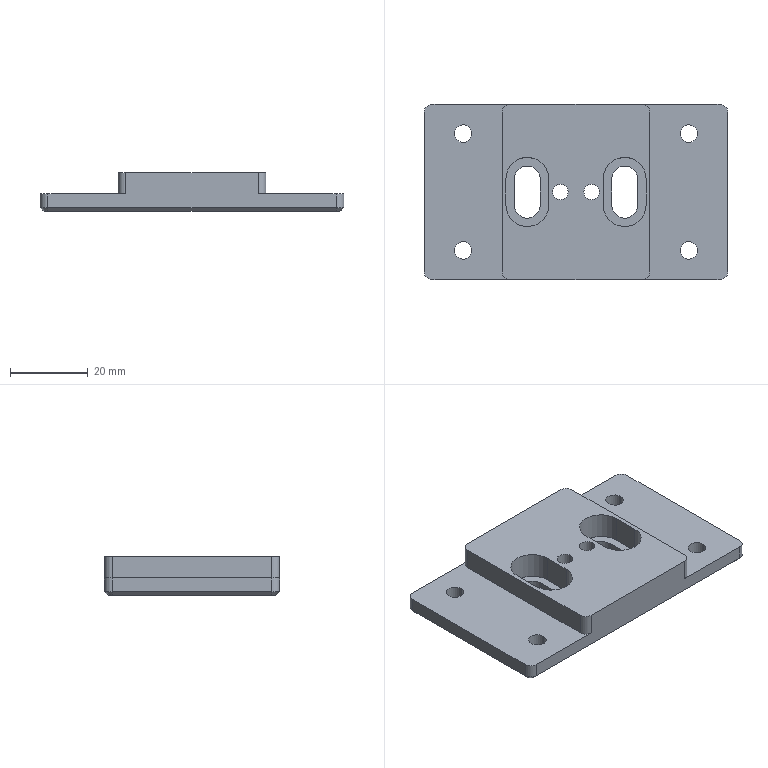NC program | NX | posted with a generic post | part box 78 x 45 x 10 mm
Lines 1683 to 3248 of 4289, first 1305 of 1562 lines:
(ZLEVEL_PROFILE_COPY_COPY_1_COPY_1 , TOOL : D6)
N3346 T06 M6
N3348 G54
N3350 G17 G0 G90 X-10.05 Y2.248 S9500 M3
N3352 G43 Z30. H6
N3354 Z1.5
N3356 G94 G1 Y3.622 Z1.428 F2200.
N3358 X-10.157 Y4.151 Z1.4
N3360 X-10.378 Y4.644 Z1.371
N3362 X-10.701 Y5.077 Z1.343
N3364 X-11.11 Y5.43 Z1.315
N3366 X-11.587 Y5.684 Z1.286
N3368 X-12.011 Y5.811 Z1.263
N3370 X-12.599 Y5.858 Z1.232
N3372 X-13.18 Y5.764 Z1.201
N3374 X-13.723 Y5.535 Z1.171
N3376 X-14.195 Y5.183 Z1.14
N3378 X-14.571 Y4.728 Z1.109
N3380 X-14.827 Y4.198 Z1.078
N3382 X-14.95 Y3.622 Z1.047
N3384 Y-3.622 Z0.667
N3386 X-14.864 Y-4.08 Z0.643
N3388 X-14.694 Y-4.514 Z0.619
N3390 X-14.458 Y-4.889 Z0.595
N3392 X-14.067 Y-5.297 Z0.566
N3394 X-13.593 Y-5.604 Z0.536
N3396 X-13.061 Y-5.795 Z0.507
N3398 X-12.5 Y-5.86 Z0.477
N3400 X-11.939 Y-5.795 Z0.447
N3402 X-11.407 Y-5.604 Z0.418
N3404 X-10.933 Y-5.297 Z0.388
N3406 X-10.542 Y-4.889 Z0.359
N3408 X-10.307 Y-4.514 Z0.335
N3410 X-10.136 Y-4.08 Z0.311
N3412 X-10.05 Y-3.622 Z0.286
N3414 Y3.622 Z-0.093
N3416 X-10.157 Y4.151 Z-0.121
N3418 X-10.378 Y4.644 Z-0.15
N3420 X-10.701 Y5.077 Z-0.178
N3422 X-11.11 Y5.43 Z-0.206
N3424 X-11.587 Y5.684 Z-0.235
N3426 X-12.011 Y5.811 Z-0.258
N3428 X-12.599 Y5.858 Z-0.289
N3430 X-13.18 Y5.764 Z-0.32
N3432 X-13.723 Y5.535 Z-0.351
N3434 X-14.195 Y5.183 Z-0.381
N3436 X-14.571 Y4.728 Z-0.412
N3438 X-14.827 Y4.198 Z-0.443
N3440 X-14.95 Y3.622 Z-0.474
N3442 Y3.4 Z-0.486
N3444 Y-3.4
N3446 G3 X-12.5 Y-5.85 R2.45
N3448 X-10.05 Y-3.4 R2.45
N3450 G1 Y3.4
N3452 G3 X-12.5 Y5.85 R2.45
N3454 X-14.95 Y3.4 R2.45
N3456 G1 Y-3.158 Z-0.632
N3458 Y-3.331 Z-0.636
N3460 X-14.94 Y-3.503 Z-0.64
N3462 X-14.929 Y-3.675 Z-0.644
N3464 X-14.901 Y-3.844 Z-0.648
N3466 X-14.865 Y-4.013 Z-0.651
N3468 X-14.816 Y-4.178 Z-0.655
N3470 X-14.754 Y-4.338 Z-0.659
N3472 X-14.686 Y-4.496 Z-0.663
N3474 X-14.6 Y-4.645 Z-0.667
N3476 X-14.508 Y-4.791 Z-0.671
N3478 X-14.406 Y-4.929 Z-0.675
N3480 X-14.292 Y-5.058 Z-0.678
N3482 X-14.174 Y-5.183 Z-0.682
N3484 X-14.042 Y-5.293 Z-0.686
N3486 X-13.905 Y-5.397 Z-0.69
N3488 X-13.761 Y-5.492 Z-0.694
N3490 X-13.61 Y-5.575 Z-0.698
N3492 X-13.455 Y-5.65 Z-0.702
N3494 X-13.294 Y-5.708 Z-0.705
N3496 X-13.129 Y-5.759 Z-0.709
N3498 X-12.962 Y-5.799 Z-0.713
N3500 X-12.792 Y-5.824 Z-0.717
N3502 X-12.621 Y-5.841 Z-0.721
N3504 X-12.449 Z-0.725
N3506 X-12.277 Y-5.832 Z-0.729
N3508 X-12.106 Y-5.812 Z-0.732
N3510 X-11.938 Y-5.775 Z-0.736
N3512 X-11.771 Y-5.733 Z-0.74
N3514 X-11.609 Y-5.674 Z-0.744
N3516 X-11.452 Y-5.605 Z-0.748
N3518 X-11.298 Y-5.528 Z-0.752
N3520 X-11.153 Y-5.436 Z-0.756
N3522 X-11.011 Y-5.338 Z-0.759
N3524 X-10.88 Y-5.227 Z-0.763
N3526 X-10.756 Y-5.108 Z-0.767
N3528 X-10.637 Y-4.983 Z-0.771
N3530 X-10.533 Y-4.846 Z-0.775
N3532 X-10.435 Y-4.705 Z-0.779
N3534 X-10.349 Y-4.556 Z-0.783
N3536 X-10.273 Y-4.402 Z-0.786
N3538 X-10.205 Y-4.244 Z-0.79
N3540 X-10.155 Y-4.079 Z-0.794
N3542 X-10.111 Y-3.912 Z-0.798
N3544 X-10.081 Y-3.743 Z-0.802
N3546 X-10.065 Y-3.572 Z-0.806
N3548 X-10.054 Y-3.4 Z-0.81
N3550 X-10.05 Y-3.227 Z-0.813
N3552 Y3.158 Z-0.956
N3554 Y3.331 Z-0.96
N3556 X-10.061 Y3.503 Z-0.964
N3558 X-10.07 Y3.675 Z-0.968
N3560 X-10.091 Y3.846 Z-0.971
N3562 G3 X-14.95 Y3.4 R2.45
N3564 G1 Y-3.158 Z-1.118
N3566 Y-3.331 Z-1.122
N3568 X-14.939 Y-3.503 Z-1.126
N3570 X-14.93 Y-3.675 Z-1.129
N3572 X-14.901 Y-3.844 Z-1.133
N3574 X-14.865 Y-4.013 Z-1.137
N3576 X-14.816 Y-4.178 Z-1.141
N3578 X-14.753 Y-4.338 Z-1.145
N3580 X-14.686 Y-4.496 Z-1.149
N3582 X-14.599 Y-4.645 Z-1.153
N3584 X-14.508 Y-4.791 Z-1.156
N3586 X-14.406 Y-4.929 Z-1.16
N3588 X-14.292 Y-5.058 Z-1.164
N3590 X-14.174 Y-5.183 Z-1.168
N3592 X-14.042 Y-5.293 Z-1.172
N3594 X-13.905 Y-5.397 Z-1.176
N3596 X-13.761 Y-5.492 Z-1.18
N3598 X-13.61 Y-5.575 Z-1.183
N3600 X-13.455 Y-5.65 Z-1.187
N3602 X-13.294 Y-5.708 Z-1.191
N3604 X-13.129 Y-5.759 Z-1.195
N3606 X-12.962 Y-5.8 Z-1.199
N3608 X-12.792 Y-5.824 Z-1.203
N3610 X-12.621 Y-5.841 Z-1.207
N3612 X-12.449 Z-1.21
N3614 X-12.277 Y-5.832 Z-1.214
N3616 X-12.106 Y-5.812 Z-1.218
N3618 X-11.938 Y-5.775 Z-1.222
N3620 X-11.771 Y-5.733 Z-1.226
N3622 X-11.609 Y-5.674 Z-1.23
N3624 X-11.452 Y-5.605 Z-1.234
N3626 X-11.298 Y-5.528 Z-1.237
N3628 X-11.153 Y-5.436 Z-1.241
N3630 X-11.011 Y-5.338 Z-1.245
N3632 X-10.88 Y-5.227 Z-1.249
N3634 X-10.756 Y-5.108 Z-1.253
N3636 X-10.637 Y-4.983 Z-1.257
N3638 X-10.533 Y-4.846 Z-1.261
N3640 X-10.435 Y-4.705 Z-1.264
N3642 X-10.349 Y-4.556 Z-1.268
N3644 X-10.273 Y-4.401 Z-1.272
N3646 X-10.205 Y-4.244 Z-1.276
N3648 X-10.155 Y-4.079 Z-1.28
N3650 X-10.111 Y-3.912 Z-1.284
N3652 X-10.081 Y-3.743 Z-1.288
N3654 X-10.065 Y-3.572 Z-1.291
N3656 X-10.054 Y-3.4 Z-1.295
N3658 X-10.05 Y-3.227 Z-1.299
N3660 Y3.158 Z-1.442
N3662 Y3.331 Z-1.446
N3664 X-10.061 Y3.503 Z-1.449
N3666 X-10.07 Y3.675 Z-1.453
N3668 X-10.091 Y3.846 Z-1.457
N3670 G3 X-14.95 Y3.4 R2.45
N3672 G1 Y-3.158 Z-1.604
N3674 Y-3.331 Z-1.607
N3676 X-14.939 Y-3.503 Z-1.611
N3678 X-14.93 Y-3.675 Z-1.615
N3680 X-14.901 Y-3.844 Z-1.619
N3682 X-14.865 Y-4.013 Z-1.623
N3684 X-14.816 Y-4.178 Z-1.627
N3686 X-14.753 Y-4.338 Z-1.631
N3688 X-14.686 Y-4.496 Z-1.634
N3690 X-14.599 Y-4.645 Z-1.638
N3692 X-14.508 Y-4.791 Z-1.642
N3694 X-14.406 Y-4.929 Z-1.646
N3696 X-14.292 Y-5.058 Z-1.65
N3698 X-14.173 Y-5.183 Z-1.654
N3700 X-14.042 Y-5.293 Z-1.658
N3702 X-13.904 Y-5.397 Z-1.661
N3704 X-13.761 Y-5.492 Z-1.665
N3706 X-13.61 Y-5.574 Z-1.669
N3708 X-13.455 Y-5.65 Z-1.673
N3710 X-13.294 Y-5.708 Z-1.677
N3712 X-13.129 Y-5.759 Z-1.681
N3714 X-12.962 Y-5.8 Z-1.685
N3716 X-12.792 Y-5.824 Z-1.688
N3718 X-12.621 Y-5.841 Z-1.692
N3720 X-12.449 Z-1.696
N3722 X-12.277 Y-5.832 Z-1.7
N3724 X-12.106 Y-5.812 Z-1.704
N3726 X-11.938 Y-5.775 Z-1.708
N3728 X-11.771 Y-5.733 Z-1.712
N3730 X-11.609 Y-5.674 Z-1.715
N3732 X-11.452 Y-5.605 Z-1.719
N3734 X-11.298 Y-5.528 Z-1.723
N3736 X-11.153 Y-5.436 Z-1.727
N3738 X-11.011 Y-5.338 Z-1.731
N3740 X-10.88 Y-5.227 Z-1.735
N3742 X-10.756 Y-5.107 Z-1.739
N3744 X-10.638 Y-4.983 Z-1.742
N3746 X-10.533 Y-4.846 Z-1.746
N3748 X-10.435 Y-4.705 Z-1.75
N3750 X-10.349 Y-4.556 Z-1.754
N3752 X-10.273 Y-4.401 Z-1.758
N3754 X-10.205 Y-4.244 Z-1.762
N3756 X-10.155 Y-4.079 Z-1.766
N3758 X-10.111 Y-3.912 Z-1.769
N3760 X-10.081 Y-3.743 Z-1.773
N3762 X-10.065 Y-3.572 Z-1.777
N3764 X-10.054 Y-3.4 Z-1.781
N3766 X-10.05 Y-3.227 Z-1.785
N3768 Y3.158 Z-1.927
N3770 Y3.331 Z-1.931
N3772 X-10.061 Y3.503 Z-1.935
N3774 X-10.071 Y3.675 Z-1.939
N3776 X-10.091 Y3.846 Z-1.943
N3778 G3 X-14.95 Y3.4 R2.45
N3780 G1 Y-3.158 Z-2.089
N3782 Y-3.331 Z-2.093
N3784 X-14.939 Y-3.503 Z-2.097
N3786 X-14.93 Y-3.675 Z-2.101
N3788 X-14.901 Y-3.844 Z-2.105
N3790 X-14.865 Y-4.013 Z-2.109
N3792 X-14.816 Y-4.178 Z-2.112
N3794 X-14.753 Y-4.338 Z-2.116
N3796 X-14.686 Y-4.496 Z-2.12
N3798 X-14.599 Y-4.645 Z-2.124
N3800 X-14.508 Y-4.791 Z-2.128
N3802 X-14.405 Y-4.929 Z-2.132
N3804 X-14.292 Y-5.058 Z-2.136
N3806 X-14.173 Y-5.183 Z-2.139
N3808 X-14.041 Y-5.293 Z-2.143
N3810 X-13.905 Y-5.398 Z-2.147
N3812 X-13.761 Y-5.492 Z-2.151
N3814 X-13.61 Y-5.574 Z-2.155
N3816 X-13.455 Y-5.65 Z-2.159
N3818 X-13.294 Y-5.709 Z-2.163
N3820 X-13.129 Y-5.759 Z-2.166
N3822 X-12.962 Y-5.799 Z-2.17
N3824 X-12.792 Y-5.824 Z-2.174
N3826 X-12.621 Y-5.841 Z-2.178
N3828 X-12.449 Z-2.182
N3830 X-12.277 Y-5.832 Z-2.186
N3832 X-12.106 Y-5.812 Z-2.19
N3834 X-11.938 Y-5.775 Z-2.193
N3836 X-11.771 Y-5.733 Z-2.197
N3838 X-11.61 Y-5.674 Z-2.201
N3840 X-11.452 Y-5.605 Z-2.205
N3842 X-11.298 Y-5.528 Z-2.209
N3844 X-11.153 Y-5.436 Z-2.213
N3846 X-11.011 Y-5.338 Z-2.217
N3848 X-10.88 Y-5.227 Z-2.22
N3850 X-10.755 Y-5.108 Z-2.224
N3852 X-10.638 Y-4.983 Z-2.228
N3854 X-10.533 Y-4.846 Z-2.232
N3856 X-10.435 Y-4.705 Z-2.236
N3858 X-10.348 Y-4.556 Z-2.24
N3860 X-10.273 Y-4.401 Z-2.244
N3862 X-10.205 Y-4.243 Z-2.247
N3864 X-10.155 Y-4.079 Z-2.251
N3866 X-10.112 Y-3.912 Z-2.255
N3868 X-10.081 Y-3.743 Z-2.259
N3870 X-10.066 Y-3.572 Z-2.263
N3872 X-10.055 Y-3.4 Z-2.267
N3874 X-10.05 Y-3.227 Z-2.271
N3876 Y3.158 Z-2.413
N3878 Y3.331 Z-2.417
N3880 X-10.061 Y3.503 Z-2.421
N3882 X-10.071 Y3.675 Z-2.425
N3884 X-10.091 Y3.846 Z-2.429
N3886 G3 X-14.95 Y3.4 R2.45
N3888 G1 Y-3.158 Z-2.575
N3890 Y-3.331 Z-2.579
N3892 X-14.939 Y-3.503 Z-2.583
N3894 X-14.929 Y-3.675 Z-2.587
N3896 X-14.901 Y-3.844 Z-2.59
N3898 X-14.865 Y-4.013 Z-2.594
N3900 X-14.816 Y-4.177 Z-2.598
N3902 X-14.754 Y-4.338 Z-2.602
N3904 X-14.686 Y-4.496 Z-2.606
N3906 X-14.599 Y-4.645 Z-2.61
N3908 X-14.508 Y-4.791 Z-2.614
N3910 X-14.405 Y-4.928 Z-2.617
N3912 X-14.292 Y-5.058 Z-2.621
N3914 X-14.173 Y-5.183 Z-2.625
N3916 X-14.041 Y-5.293 Z-2.629
N3918 X-13.905 Y-5.398 Z-2.633
N3920 X-13.761 Y-5.492 Z-2.637
N3922 X-13.61 Y-5.574 Z-2.641
N3924 X-13.455 Y-5.65 Z-2.644
N3926 X-13.294 Y-5.709 Z-2.648
N3928 X-13.129 Y-5.759 Z-2.652
N3930 X-12.962 Y-5.799 Z-2.656
N3932 X-12.792 Y-5.824 Z-2.66
N3934 X-12.621 Y-5.84 Z-2.664
N3936 X-12.449 Y-5.841 Z-2.668
N3938 X-12.277 Y-5.832 Z-2.671
N3940 X-12.106 Y-5.812 Z-2.675
N3942 X-11.938 Y-5.775 Z-2.679
N3944 X-11.771 Y-5.733 Z-2.683
N3946 X-11.61 Y-5.674 Z-2.687
N3948 X-11.452 Y-5.605 Z-2.691
N3950 X-11.298 Y-5.527 Z-2.695
N3952 X-11.153 Y-5.436 Z-2.698
N3954 X-11.012 Y-5.338 Z-2.702
N3956 X-10.88 Y-5.226 Z-2.706
N3958 X-10.755 Y-5.108 Z-2.71
N3960 X-10.638 Y-4.983 Z-2.714
N3962 X-10.533 Y-4.846 Z-2.718
N3964 X-10.435 Y-4.705 Z-2.722
N3966 X-10.348 Y-4.556 Z-2.725
N3968 X-10.274 Y-4.401 Z-2.729
N3970 X-10.205 Y-4.243 Z-2.733
N3972 X-10.155 Y-4.079 Z-2.737
N3974 X-10.112 Y-3.912 Z-2.741
N3976 X-10.082 Y-3.743 Z-2.745
N3978 X-10.064 Y-3.572 Z-2.749
N3980 X-10.055 Y-3.4 Z-2.752
N3982 X-10.05 Y-3.227 Z-2.756
N3984 Y3.158 Z-2.899
N3986 Y3.331 Z-2.903
N3988 X-10.061 Y3.503 Z-2.907
N3990 X-10.071 Y3.675 Z-2.91
N3992 X-10.091 Y3.846 Z-2.914
N3994 G3 X-14.95 Y3.4 R2.45
N3996 G1 Y-3.158 Z-3.061
N3998 Y-3.331 Z-3.065
N4000 X-14.939 Y-3.503 Z-3.068
N4002 X-14.929 Y-3.675 Z-3.072
N4004 X-14.9 Y-3.844 Z-3.076
N4006 X-14.864 Y-4.013 Z-3.08
N4008 X-14.816 Y-4.177 Z-3.084
N4010 X-14.754 Y-4.338 Z-3.088
N4012 X-14.686 Y-4.496 Z-3.092
N4014 X-14.6 Y-4.645 Z-3.095
N4016 X-14.508 Y-4.791 Z-3.099
N4018 X-14.405 Y-4.928 Z-3.103
N4020 X-14.292 Y-5.058 Z-3.107
N4022 X-14.173 Y-5.182 Z-3.111
N4024 X-14.041 Y-5.293 Z-3.115
N4026 X-13.905 Y-5.398 Z-3.119
N4028 X-13.761 Y-5.492 Z-3.122
N4030 X-13.61 Y-5.574 Z-3.126
N4032 X-13.455 Y-5.649 Z-3.13
N4034 X-13.294 Y-5.709 Z-3.134
N4036 X-13.129 Y-5.759 Z-3.138
N4038 X-12.962 Y-5.799 Z-3.142
N4040 X-12.792 Y-5.824 Z-3.146
N4042 X-12.621 Y-5.84 Z-3.149
N4044 X-12.449 Y-5.841 Z-3.153
N4046 X-12.277 Y-5.831 Z-3.157
N4048 X-12.106 Y-5.812 Z-3.161
N4050 X-11.938 Y-5.774 Z-3.165
N4052 X-11.771 Y-5.733 Z-3.169
N4054 X-11.61 Y-5.673 Z-3.173
N4056 X-11.452 Y-5.605 Z-3.176
N4058 X-11.298 Y-5.527 Z-3.18
N4060 X-11.153 Y-5.436 Z-3.184
N4062 X-11.012 Y-5.337 Z-3.188
N4064 X-10.88 Y-5.226 Z-3.192
N4066 X-10.755 Y-5.108 Z-3.196
N4068 X-10.638 Y-4.983 Z-3.2
N4070 X-10.534 Y-4.846 Z-3.203
N4072 X-10.435 Y-4.705 Z-3.207
N4074 X-10.349 Y-4.556 Z-3.211
N4076 X-10.274 Y-4.401 Z-3.215
N4078 X-10.205 Y-4.243 Z-3.219
N4080 X-10.155 Y-4.079 Z-3.223
N4082 X-10.112 Y-3.912 Z-3.227
N4084 X-10.082 Y-3.743 Z-3.23
N4086 X-10.065 Y-3.572 Z-3.234
N4088 X-10.055 Y-3.4 Z-3.238
N4090 X-10.05 Y-3.227 Z-3.242
N4092 Y3.158 Z-3.385
N4094 Y3.331 Z-3.388
N4096 X-10.061 Y3.503 Z-3.392
N4098 X-10.071 Y3.675 Z-3.396
N4100 X-10.091 Y3.846 Z-3.4
N4102 G3 X-14.95 Y3.4 R2.45
N4104 G1 Y-3.158 Z-3.546
N4106 Y-3.331 Z-3.55
N4108 X-14.939 Y-3.503 Z-3.554
N4110 X-14.929 Y-3.675 Z-3.558
N4112 X-14.9 Y-3.844 Z-3.562
N4114 X-14.864 Y-4.012 Z-3.566
N4116 X-14.815 Y-4.177 Z-3.57
N4118 X-14.754 Y-4.338 Z-3.573
N4120 X-14.686 Y-4.496 Z-3.577
N4122 X-14.6 Y-4.645 Z-3.581
N4124 X-14.508 Y-4.791 Z-3.585
N4126 X-14.405 Y-4.928 Z-3.589
N4128 X-14.292 Y-5.058 Z-3.593
N4130 X-14.173 Y-5.182 Z-3.597
N4132 X-14.041 Y-5.293 Z-3.6
N4134 X-13.905 Y-5.398 Z-3.604
N4136 X-13.761 Y-5.492 Z-3.608
N4138 X-13.61 Y-5.574 Z-3.612
N4140 X-13.455 Y-5.649 Z-3.616
N4142 X-13.294 Y-5.709 Z-3.62
N4144 X-13.129 Y-5.759 Z-3.624
N4146 X-12.962 Y-5.799 Z-3.627
N4148 X-12.792 Y-5.824 Z-3.631
N4150 X-12.621 Y-5.84 Z-3.635
N4152 X-12.449 Y-5.841 Z-3.639
N4154 X-12.277 Y-5.831 Z-3.643
N4156 X-12.106 Y-5.812 Z-3.647
N4158 X-11.938 Y-5.776 Z-3.651
N4160 X-11.771 Y-5.733 Z-3.654
N4162 X-11.61 Y-5.673 Z-3.658
N4164 X-11.452 Y-5.605 Z-3.662
N4166 X-11.299 Y-5.527 Z-3.666
N4168 X-11.153 Y-5.436 Z-3.67
N4170 X-11.012 Y-5.337 Z-3.674
N4172 X-10.88 Y-5.226 Z-3.678
N4174 X-10.756 Y-5.108 Z-3.681
N4176 X-10.638 Y-4.983 Z-3.685
N4178 X-10.534 Y-4.846 Z-3.689
N4180 X-10.435 Y-4.705 Z-3.693
N4182 X-10.349 Y-4.556 Z-3.697
N4184 X-10.274 Y-4.401 Z-3.701
N4186 X-10.206 Y-4.243 Z-3.705
N4188 X-10.155 Y-4.079 Z-3.708
N4190 X-10.112 Y-3.912 Z-3.712
N4192 X-10.082 Y-3.743 Z-3.716
N4194 X-10.065 Y-3.572 Z-3.72
N4196 X-10.055 Y-3.4 Z-3.724
N4198 X-10.05 Y-3.227 Z-3.728
N4200 Y3.158 Z-3.87
N4202 Y3.331 Z-3.874
N4204 X-10.061 Y3.503 Z-3.878
N4206 X-10.071 Y3.675 Z-3.882
N4208 X-10.091 Y3.846 Z-3.886
N4210 G3 X-14.95 Y3.4 R2.45
N4212 G1 Y-3.158 Z-4.032
N4214 Y-3.331 Z-4.036
N4216 X-14.939 Y-3.503 Z-4.04
N4218 X-14.929 Y-3.675 Z-4.044
N4220 X-14.9 Y-3.844 Z-4.048
N4222 X-14.864 Y-4.012 Z-4.051
N4224 X-14.815 Y-4.177 Z-4.055
N4226 X-14.754 Y-4.338 Z-4.059
N4228 X-14.686 Y-4.496 Z-4.063
N4230 X-14.6 Y-4.645 Z-4.067
N4232 X-14.508 Y-4.791 Z-4.071
N4234 X-14.405 Y-4.928 Z-4.075
N4236 X-14.292 Y-5.058 Z-4.078
N4238 X-14.173 Y-5.182 Z-4.082
N4240 X-14.041 Y-5.293 Z-4.086
N4242 X-13.905 Y-5.398 Z-4.09
N4244 X-13.761 Y-5.492 Z-4.094
N4246 X-13.61 Y-5.574 Z-4.098
N4248 X-13.455 Y-5.649 Z-4.102
N4250 X-13.294 Y-5.709 Z-4.105
N4252 X-13.129 Y-5.759 Z-4.109
N4254 X-12.962 Y-5.799 Z-4.113
N4256 X-12.792 Y-5.823 Z-4.117
N4258 X-12.621 Y-5.84 Z-4.121
N4260 X-12.449 Z-4.125
N4262 X-12.277 Y-5.831 Z-4.129
N4264 X-12.106 Y-5.812 Z-4.132
N4266 X-11.938 Y-5.775 Z-4.136
N4268 X-11.771 Y-5.732 Z-4.14
N4270 X-11.61 Y-5.673 Z-4.144
N4272 X-11.452 Y-5.605 Z-4.148
N4274 X-11.299 Y-5.527 Z-4.152
N4276 X-11.153 Y-5.436 Z-4.156
N4278 X-11.012 Y-5.337 Z-4.159
N4280 X-10.88 Y-5.226 Z-4.163
N4282 X-10.756 Y-5.108 Z-4.167
N4284 X-10.638 Y-4.983 Z-4.171
N4286 X-10.534 Y-4.846 Z-4.175
N4288 X-10.435 Y-4.705 Z-4.179
N4290 X-10.349 Y-4.556 Z-4.183
N4292 X-10.274 Y-4.401 Z-4.186
N4294 X-10.206 Y-4.243 Z-4.19
N4296 X-10.155 Y-4.079 Z-4.194
N4298 X-10.112 Y-3.912 Z-4.198
N4300 X-10.082 Y-3.743 Z-4.202
N4302 X-10.065 Y-3.572 Z-4.206
N4304 X-10.055 Y-3.4 Z-4.21
N4306 X-10.05 Y-3.227 Z-4.213
N4308 Y3.158 Z-4.356
N4310 Y3.331 Z-4.36
N4312 X-10.061 Y3.503 Z-4.364
N4314 X-10.071 Y3.675 Z-4.368
N4316 X-10.091 Y3.846 Z-4.371
N4318 G3 X-14.95 Y3.4 R2.45
N4320 G1 Y-3.158 Z-4.518
N4322 Y-3.331 Z-4.522
N4324 X-14.939 Y-3.503 Z-4.526
N4326 X-14.929 Y-3.675 Z-4.529
N4328 X-14.9 Y-3.844 Z-4.533
N4330 X-14.864 Y-4.012 Z-4.537
N4332 X-14.815 Y-4.177 Z-4.541
N4334 X-14.754 Y-4.338 Z-4.545
N4336 X-14.686 Y-4.496 Z-4.549
N4338 X-14.6 Y-4.645 Z-4.553
N4340 X-14.508 Y-4.79 Z-4.556
N4342 X-14.405 Y-4.928 Z-4.56
N4344 X-14.292 Y-5.058 Z-4.564
N4346 X-14.173 Y-5.182 Z-4.568
N4348 X-14.041 Y-5.293 Z-4.572
N4350 X-13.905 Y-5.397 Z-4.576
N4352 X-13.761 Y-5.492 Z-4.58
N4354 X-13.609 Y-5.573 Z-4.583
N4356 X-13.455 Y-5.649 Z-4.587
N4358 X-13.294 Y-5.708 Z-4.591
N4360 X-13.129 Y-5.758 Z-4.595
N4362 X-12.962 Y-5.798 Z-4.599
N4364 X-12.792 Y-5.823 Z-4.603
N4366 X-12.621 Y-5.841 Z-4.607
N4368 X-12.449 Y-5.84 Z-4.61
N4370 X-12.277 Y-5.831 Z-4.614
N4372 X-12.106 Y-5.812 Z-4.618
N4374 X-11.938 Y-5.775 Z-4.622
N4376 X-11.771 Y-5.732 Z-4.626
N4378 X-11.61 Y-5.673 Z-4.63
N4380 X-11.452 Y-5.604 Z-4.634
N4382 X-11.298 Y-5.528 Z-4.637
N4384 X-11.153 Y-5.436 Z-4.641
N4386 X-11.012 Y-5.337 Z-4.645
N4388 X-10.88 Y-5.226 Z-4.649
N4390 X-10.756 Y-5.108 Z-4.653
N4392 X-10.638 Y-4.982 Z-4.657
N4394 X-10.534 Y-4.846 Z-4.661
N4396 X-10.435 Y-4.705 Z-4.664
N4398 X-10.349 Y-4.556 Z-4.668
N4400 X-10.274 Y-4.401 Z-4.672
N4402 X-10.206 Y-4.243 Z-4.676
N4404 X-10.155 Y-4.079 Z-4.68
N4406 X-10.113 Y-3.912 Z-4.684
N4408 X-10.082 Y-3.743 Z-4.688
N4410 X-10.065 Y-3.572 Z-4.691
N4412 X-10.055 Y-3.4 Z-4.695
N4414 X-10.05 Y-3.227 Z-4.699
N4416 Y3.158 Z-4.842
N4418 Y3.331 Z-4.846
N4420 X-10.061 Y3.503 Z-4.849
N4422 X-10.071 Y3.675 Z-4.853
N4424 X-10.091 Y3.846 Z-4.857
N4426 G3 X-14.95 Y3.4 R2.45
N4428 G1 Y-3.158 Z-5.004
N4430 Y-3.331 Z-5.007
N4432 X-14.939 Y-3.503 Z-5.011
N4434 X-14.928 Y-3.675 Z-5.015
N4436 X-14.9 Y-3.844 Z-5.019
N4438 X-14.864 Y-4.012 Z-5.023
N4440 X-14.815 Y-4.177 Z-5.027
N4442 X-14.753 Y-4.338 Z-5.031
N4444 X-14.686 Y-4.496 Z-5.034
N4446 X-14.599 Y-4.645 Z-5.038
N4448 X-14.508 Y-4.79 Z-5.042
N4450 X-14.404 Y-4.928 Z-5.046
N4452 X-14.292 Y-5.058 Z-5.05
N4454 X-14.173 Y-5.182 Z-5.054
N4456 X-14.041 Y-5.293 Z-5.058
N4458 X-13.904 Y-5.397 Z-5.061
N4460 X-13.761 Y-5.492 Z-5.065
N4462 X-13.609 Y-5.573 Z-5.069
N4464 X-13.455 Y-5.649 Z-5.073
N4466 X-13.294 Y-5.708 Z-5.077
N4468 X-13.129 Y-5.758 Z-5.081
N4470 X-12.962 Y-5.798 Z-5.085
N4472 X-12.792 Y-5.823 Z-5.088
N4474 X-12.621 Y-5.841 Z-5.092
N4476 X-12.449 Y-5.84 Z-5.096
N4478 X-12.277 Y-5.831 Z-5.1
N4480 X-12.106 Y-5.812 Z-5.104
N4482 X-11.938 Y-5.775 Z-5.108
N4484 X-11.771 Y-5.732 Z-5.112
N4486 X-11.61 Y-5.673 Z-5.115
N4488 X-11.452 Y-5.604 Z-5.119
N4490 X-11.298 Y-5.528 Z-5.123
N4492 X-11.153 Y-5.435 Z-5.127
N4494 X-11.012 Y-5.337 Z-5.131
N4496 X-10.881 Y-5.226 Z-5.135
N4498 X-10.756 Y-5.108 Z-5.139
N4500 X-10.638 Y-4.982 Z-5.142
N4502 X-10.534 Y-4.845 Z-5.146
N4504 X-10.435 Y-4.705 Z-5.15
N4506 X-10.349 Y-4.556 Z-5.154
N4508 X-10.274 Y-4.401 Z-5.158
N4510 X-10.206 Y-4.243 Z-5.162
N4512 X-10.155 Y-4.079 Z-5.166
N4514 X-10.113 Y-3.912 Z-5.169
N4516 X-10.082 Y-3.743 Z-5.173
N4518 X-10.065 Y-3.572 Z-5.177
N4520 X-10.055 Y-3.4 Z-5.181
N4522 X-10.05 Y-3.227 Z-5.185
N4524 Y3.158 Z-5.327
N4526 Y3.331 Z-5.331
N4528 X-10.061 Y3.503 Z-5.335
N4530 X-10.072 Y3.675 Z-5.339
N4532 X-10.091 Y3.846 Z-5.343
N4534 G3 X-14.95 Y3.4 R2.45
N4536 G1 Y-3.158 Z-5.489
N4538 Y-3.331 Z-5.493
N4540 X-14.939 Y-3.503 Z-5.497
N4542 X-14.928 Y-3.675 Z-5.501
N4544 X-14.9 Y-3.844 Z-5.505
N4546 X-14.863 Y-4.012 Z-5.509
N4548 X-14.815 Y-4.177 Z-5.512
N4550 X-14.753 Y-4.338 Z-5.516
N4552 X-14.685 Y-4.496 Z-5.52
N4554 X-14.599 Y-4.645 Z-5.524
N4556 X-14.508 Y-4.79 Z-5.528
N4558 X-14.404 Y-4.928 Z-5.532
N4560 X-14.292 Y-5.058 Z-5.536
N4562 X-14.172 Y-5.182 Z-5.539
N4564 X-14.041 Y-5.293 Z-5.543
N4566 X-13.904 Y-5.397 Z-5.547
N4568 X-13.761 Y-5.491 Z-5.551
N4570 X-13.609 Y-5.573 Z-5.555
N4572 X-13.455 Y-5.649 Z-5.559
N4574 X-13.294 Y-5.708 Z-5.563
N4576 X-13.129 Y-5.758 Z-5.566
N4578 X-12.962 Y-5.798 Z-5.57
N4580 X-12.792 Y-5.823 Z-5.574
N4582 X-12.621 Y-5.841 Z-5.578
N4584 X-12.449 Y-5.84 Z-5.582
N4586 X-12.277 Y-5.83 Z-5.586
N4588 X-12.106 Y-5.811 Z-5.59
N4590 X-11.938 Y-5.775 Z-5.593
N4592 X-11.771 Y-5.732 Z-5.597
N4594 X-11.61 Y-5.673 Z-5.601
N4596 X-11.452 Y-5.604 Z-5.605
N4598 X-11.298 Y-5.528 Z-5.609
N4600 X-11.153 Y-5.435 Z-5.613
N4602 X-11.012 Y-5.337 Z-5.617
N4604 X-10.881 Y-5.226 Z-5.62
N4606 X-10.756 Y-5.107 Z-5.624
N4608 X-10.638 Y-4.982 Z-5.628
N4610 X-10.534 Y-4.845 Z-5.632
N4612 X-10.436 Y-4.704 Z-5.636
N4614 X-10.349 Y-4.556 Z-5.64
N4616 X-10.274 Y-4.401 Z-5.644
N4618 X-10.206 Y-4.243 Z-5.647
N4620 X-10.156 Y-4.079 Z-5.651
N4622 X-10.113 Y-3.912 Z-5.655
N4624 X-10.082 Y-3.743 Z-5.659
N4626 X-10.066 Y-3.572 Z-5.663
N4628 X-10.055 Y-3.4 Z-5.667
N4630 X-10.05 Y-3.227 Z-5.671
N4632 Y3.158 Z-5.813
N4634 Y3.331 Z-5.817
N4636 X-10.062 Y3.503 Z-5.821
N4638 X-10.072 Y3.675 Z-5.825
N4640 X-10.091 Y3.846 Z-5.829
N4642 G3 X-14.95 Y3.4 R2.45
N4644 G1 Y-3.158 Z-5.975
N4646 Y-3.331 Z-5.979
N4648 X-14.938 Y-3.503 Z-5.983
N4650 X-14.928 Y-3.675 Z-5.987
N4652 X-14.9 Y-3.844 Z-5.99
N4654 X-14.863 Y-4.012 Z-5.994
N4656 X-14.815 Y-4.177 Z-5.998
N4658 X-14.753 Y-4.338 Z-6.002
N4660 X-14.685 Y-4.496 Z-6.006
N4662 X-14.599 Y-4.645 Z-6.01
N4664 X-14.508 Y-4.79 Z-6.014
N4666 X-14.404 Y-4.928 Z-6.017
N4668 X-14.291 Y-5.057 Z-6.021
N4670 X-14.172 Y-5.182 Z-6.025
N4672 X-14.041 Y-5.293 Z-6.029
N4674 X-13.904 Y-5.397 Z-6.033
N4676 X-13.761 Y-5.491 Z-6.037
N4678 X-13.609 Y-5.573 Z-6.041
N4680 X-13.455 Y-5.649 Z-6.044
N4682 X-13.294 Y-5.708 Z-6.048
N4684 X-13.129 Y-5.758 Z-6.052
N4686 X-12.962 Y-5.798 Z-6.056
N4688 X-12.792 Y-5.823 Z-6.06
N4690 X-12.621 Y-5.84 Z-6.064
N4692 X-12.449 Z-6.068
N4694 X-12.277 Y-5.83 Z-6.071
N4696 X-12.106 Y-5.811 Z-6.075
N4698 X-11.938 Y-5.775 Z-6.079
N4700 X-11.771 Y-5.732 Z-6.083
N4702 X-11.61 Y-5.672 Z-6.087
N4704 X-11.452 Y-5.604 Z-6.091
N4706 X-11.298 Y-5.527 Z-6.095
N4708 X-11.153 Y-5.435 Z-6.098
N4710 X-11.012 Y-5.337 Z-6.102
N4712 X-10.881 Y-5.226 Z-6.106
N4714 X-10.756 Y-5.107 Z-6.11
N4716 X-10.638 Y-4.982 Z-6.114
N4718 X-10.534 Y-4.845 Z-6.118
N4720 X-10.436 Y-4.704 Z-6.122
N4722 X-10.35 Y-4.556 Z-6.125
N4724 X-10.274 Y-4.401 Z-6.129
N4726 X-10.207 Y-4.243 Z-6.133
N4728 X-10.156 Y-4.079 Z-6.137
N4730 X-10.113 Y-3.912 Z-6.141
N4732 X-10.082 Y-3.743 Z-6.145
N4734 X-10.066 Y-3.572 Z-6.149
N4736 X-10.055 Y-3.4 Z-6.152
N4738 X-10.05 Y-3.227 Z-6.156
N4740 Y3.158 Z-6.299
N4742 Y3.331 Z-6.303
N4744 X-10.062 Y3.503 Z-6.307
N4746 X-10.072 Y3.675 Z-6.31
N4748 X-10.091 Y3.846 Z-6.314
N4750 G3 X-14.95 Y3.4 R2.45
N4752 G1 Y-3.158 Z-6.461
N4754 Y-3.331 Z-6.465
N4756 X-14.938 Y-3.503 Z-6.468
N4758 X-14.928 Y-3.675 Z-6.472
N4760 X-14.9 Y-3.844 Z-6.476
N4762 X-14.863 Y-4.012 Z-6.48
N4764 X-14.815 Y-4.177 Z-6.484
N4766 X-14.753 Y-4.338 Z-6.488
N4768 X-14.685 Y-4.496 Z-6.492
N4770 X-14.599 Y-4.645 Z-6.495
N4772 X-14.507 Y-4.79 Z-6.499
N4774 X-14.404 Y-4.928 Z-6.503
N4776 X-14.291 Y-5.057 Z-6.507
N4778 X-14.172 Y-5.181 Z-6.511
N4780 X-14.041 Y-5.293 Z-6.515
N4782 X-13.904 Y-5.397 Z-6.519
N4784 X-13.761 Y-5.491 Z-6.522
N4786 X-13.609 Y-5.573 Z-6.526
N4788 X-13.455 Y-5.649 Z-6.53
N4790 X-13.293 Y-5.708 Z-6.534
N4792 X-13.129 Y-5.758 Z-6.538
N4794 X-12.962 Y-5.798 Z-6.542
N4796 X-12.792 Y-5.823 Z-6.546
N4798 X-12.621 Y-5.84 Z-6.549
N4800 X-12.449 Z-6.553
N4802 X-12.277 Y-5.83 Z-6.557
N4804 X-12.106 Y-5.811 Z-6.561
N4806 X-11.938 Y-5.775 Z-6.565
N4808 X-11.771 Y-5.732 Z-6.569
N4810 X-11.61 Y-5.672 Z-6.573
N4812 X-11.452 Y-5.604 Z-6.576
N4814 X-11.298 Y-5.527 Z-6.58
N4816 X-11.153 Y-5.435 Z-6.584
N4818 X-11.012 Y-5.336 Z-6.588
N4820 X-10.881 Y-5.226 Z-6.592
N4822 X-10.756 Y-5.107 Z-6.596
N4824 X-10.638 Y-4.982 Z-6.6
N4826 X-10.535 Y-4.845 Z-6.603
N4828 X-10.436 Y-4.704 Z-6.607
N4830 X-10.35 Y-4.555 Z-6.611
N4832 X-10.274 Y-4.401 Z-6.615
N4834 X-10.207 Y-4.243 Z-6.619
N4836 X-10.156 Y-4.079 Z-6.623
N4838 X-10.113 Y-3.912 Z-6.627
N4840 X-10.082 Y-3.743 Z-6.63
N4842 X-10.066 Y-3.572 Z-6.634
N4844 X-10.055 Y-3.4 Z-6.638
N4846 X-10.05 Y-3.227 Z-6.642
N4848 Y3.158 Z-6.785
N4850 Y3.331 Z-6.788
N4852 X-10.062 Y3.503 Z-6.792
N4854 X-10.072 Y3.675 Z-6.796
N4856 X-10.091 Y3.846 Z-6.8
N4858 G3 X-14.95 Y3.4 R2.45
N4860 G1 Y-3.4
N4862 G3 X-12.5 Y-5.85 R2.45
N4864 X-10.05 Y-3.4 R2.45
N4866 G1 Y3.4
N4868 G3 X-10.091 Y3.846 R2.45
N4870 X-10.48 Y4.302 R0.6
N4872 G1 X-10.845 Y4.432
N4874 Z-6.2
N4876 G0 Z30.
N4878 X14.95 Y2.248
N4880 Z1.5
N4882 G1 Y3.622 Z1.428
N4884 X14.843 Y4.151 Z1.4
N4886 X14.622 Y4.644 Z1.371
N4888 X14.299 Y5.077 Z1.343
N4890 X13.89 Y5.43 Z1.315
N4892 X13.413 Y5.684 Z1.286
N4894 X12.989 Y5.811 Z1.263
N4896 X12.401 Y5.858 Z1.232
N4898 X11.82 Y5.764 Z1.201
N4900 X11.277 Y5.535 Z1.171
N4902 X10.805 Y5.183 Z1.14
N4904 X10.429 Y4.728 Z1.109
N4906 X10.173 Y4.198 Z1.078
N4908 X10.05 Y3.622 Z1.047
N4910 Y-3.622 Z0.667
N4912 X10.136 Y-4.08 Z0.643
N4914 X10.307 Y-4.514 Z0.619
N4916 X10.542 Y-4.889 Z0.595
N4918 X10.933 Y-5.297 Z0.566
N4920 X11.407 Y-5.604 Z0.536
N4922 X11.939 Y-5.795 Z0.507
N4924 X12.5 Y-5.86 Z0.477
N4926 X13.061 Y-5.795 Z0.447
N4928 X13.593 Y-5.604 Z0.418
N4930 X14.067 Y-5.297 Z0.388
N4932 X14.458 Y-4.889 Z0.359
N4934 X14.694 Y-4.514 Z0.335
N4936 X14.864 Y-4.08 Z0.311
N4938 X14.95 Y-3.622 Z0.286
N4940 Y3.622 Z-0.093
N4942 X14.843 Y4.151 Z-0.121
N4944 X14.622 Y4.644 Z-0.15
N4946 X14.299 Y5.077 Z-0.178
N4948 X13.89 Y5.43 Z-0.206
N4950 X13.413 Y5.684 Z-0.235
N4952 X12.989 Y5.811 Z-0.258
N4954 X12.401 Y5.858 Z-0.289
N4956 X11.82 Y5.764 Z-0.32
N4958 X11.277 Y5.535 Z-0.351
N4960 X10.805 Y5.183 Z-0.381
N4962 X10.429 Y4.728 Z-0.412
N4964 X10.173 Y4.198 Z-0.443
N4966 X10.05 Y3.622 Z-0.474
N4968 Y3.4 Z-0.486
N4970 Y-3.4
N4972 G3 X12.5 Y-5.85 R2.45
N4974 X14.95 Y-3.4 R2.45
N4976 G1 Y3.4
N4978 G3 X12.5 Y5.85 R2.45
N4980 X10.05 Y3.4 R2.45
N4982 G1 Y-3.158 Z-0.632
N4984 Y-3.331 Z-0.636
N4986 X10.06 Y-3.503 Z-0.64
N4988 X10.071 Y-3.675 Z-0.644
N4990 X10.099 Y-3.844 Z-0.648
N4992 X10.135 Y-4.013 Z-0.651
N4994 X10.184 Y-4.178 Z-0.655
N4996 X10.246 Y-4.338 Z-0.659
N4998 X10.314 Y-4.496 Z-0.663
N5000 X10.4 Y-4.645 Z-0.667
N5002 X10.492 Y-4.791 Z-0.671
N5004 X10.594 Y-4.929 Z-0.675
N5006 X10.708 Y-5.058 Z-0.678
N5008 X10.826 Y-5.183 Z-0.682
N5010 X10.958 Y-5.293 Z-0.686
N5012 X11.095 Y-5.397 Z-0.69
N5014 X11.239 Y-5.492 Z-0.694
N5016 X11.39 Y-5.575 Z-0.698
N5018 X11.545 Y-5.65 Z-0.702
N5020 X11.706 Y-5.708 Z-0.705
N5022 X11.871 Y-5.759 Z-0.709
N5024 X12.038 Y-5.799 Z-0.713
N5026 X12.208 Y-5.824 Z-0.717
N5028 X12.379 Y-5.841 Z-0.721
N5030 X12.551 Z-0.725
N5032 X12.723 Y-5.832 Z-0.729
N5034 X12.894 Y-5.812 Z-0.732
N5036 X13.062 Y-5.775 Z-0.736
N5038 X13.229 Y-5.733 Z-0.74
N5040 X13.391 Y-5.674 Z-0.744
N5042 X13.548 Y-5.605 Z-0.748
N5044 X13.702 Y-5.528 Z-0.752
N5046 X13.847 Y-5.436 Z-0.756
N5048 X13.989 Y-5.338 Z-0.759
N5050 X14.12 Y-5.227 Z-0.763
N5052 X14.244 Y-5.108 Z-0.767
N5054 X14.363 Y-4.983 Z-0.771
N5056 X14.467 Y-4.846 Z-0.775
N5058 X14.565 Y-4.705 Z-0.779
N5060 X14.651 Y-4.556 Z-0.783
N5062 X14.727 Y-4.402 Z-0.786
N5064 X14.795 Y-4.244 Z-0.79
N5066 X14.845 Y-4.079 Z-0.794
N5068 X14.889 Y-3.912 Z-0.798
N5070 X14.919 Y-3.743 Z-0.802
N5072 X14.935 Y-3.572 Z-0.806
N5074 X14.946 Y-3.4 Z-0.81
N5076 X14.95 Y-3.227 Z-0.813
N5078 Y3.158 Z-0.956
N5080 Y3.331 Z-0.96
N5082 X14.939 Y3.503 Z-0.964
N5084 X14.93 Y3.675 Z-0.968
N5086 X14.909 Y3.846 Z-0.971
N5088 G3 X10.05 Y3.4 R2.45
N5090 G1 Y-3.158 Z-1.118
N5092 Y-3.331 Z-1.122
N5094 X10.061 Y-3.503 Z-1.126
N5096 X10.07 Y-3.675 Z-1.129
N5098 X10.099 Y-3.844 Z-1.133
N5100 X10.135 Y-4.013 Z-1.137
N5102 X10.184 Y-4.178 Z-1.141
N5104 X10.247 Y-4.338 Z-1.145
N5106 X10.314 Y-4.496 Z-1.149
N5108 X10.401 Y-4.645 Z-1.153
N5110 X10.492 Y-4.791 Z-1.156
N5112 X10.594 Y-4.929 Z-1.16
N5114 X10.708 Y-5.058 Z-1.164
N5116 X10.826 Y-5.183 Z-1.168
N5118 X10.958 Y-5.293 Z-1.172
N5120 X11.095 Y-5.397 Z-1.176
N5122 X11.239 Y-5.492 Z-1.18
N5124 X11.39 Y-5.575 Z-1.183
N5126 X11.545 Y-5.65 Z-1.187
N5128 X11.706 Y-5.708 Z-1.191
N5130 X11.871 Y-5.759 Z-1.195
N5132 X12.038 Y-5.8 Z-1.199
N5134 X12.208 Y-5.824 Z-1.203
N5136 X12.379 Y-5.841 Z-1.207
N5138 X12.551 Z-1.21
N5140 X12.723 Y-5.832 Z-1.214
N5142 X12.894 Y-5.812 Z-1.218
N5144 X13.062 Y-5.775 Z-1.222
N5146 X13.229 Y-5.733 Z-1.226
N5148 X13.391 Y-5.674 Z-1.23
N5150 X13.548 Y-5.605 Z-1.234
N5152 X13.702 Y-5.528 Z-1.237
N5154 X13.847 Y-5.436 Z-1.241
N5156 X13.989 Y-5.338 Z-1.245
N5158 X14.12 Y-5.227 Z-1.249
N5160 X14.244 Y-5.108 Z-1.253
N5162 X14.363 Y-4.983 Z-1.257
N5164 X14.467 Y-4.846 Z-1.261
N5166 X14.565 Y-4.705 Z-1.264
N5168 X14.651 Y-4.556 Z-1.268
N5170 X14.727 Y-4.401 Z-1.272
N5172 X14.795 Y-4.244 Z-1.276
N5174 X14.845 Y-4.079 Z-1.28
N5176 X14.889 Y-3.912 Z-1.284
N5178 X14.919 Y-3.743 Z-1.288
N5180 X14.935 Y-3.572 Z-1.291
N5182 X14.946 Y-3.4 Z-1.295
N5184 X14.95 Y-3.227 Z-1.299
N5186 Y3.158 Z-1.442
N5188 Y3.331 Z-1.446
N5190 X14.939 Y3.503 Z-1.449
N5192 X14.93 Y3.675 Z-1.453
N5194 X14.909 Y3.846 Z-1.457
N5196 G3 X10.05 Y3.4 R2.45
N5198 G1 Y-3.158 Z-1.604
N5200 Y-3.331 Z-1.607
N5202 X10.061 Y-3.503 Z-1.611
N5204 X10.07 Y-3.675 Z-1.615
N5206 X10.099 Y-3.844 Z-1.619
N5208 X10.135 Y-4.013 Z-1.623
N5210 X10.184 Y-4.178 Z-1.627
N5212 X10.247 Y-4.338 Z-1.631
N5214 X10.314 Y-4.496 Z-1.634
N5216 X10.401 Y-4.645 Z-1.638
N5218 X10.492 Y-4.791 Z-1.642
N5220 X10.594 Y-4.929 Z-1.646
N5222 X10.708 Y-5.058 Z-1.65
N5224 X10.827 Y-5.183 Z-1.654
N5226 X10.958 Y-5.293 Z-1.658
N5228 X11.096 Y-5.397 Z-1.661
N5230 X11.239 Y-5.492 Z-1.665
N5232 X11.39 Y-5.574 Z-1.669
N5234 X11.545 Y-5.65 Z-1.673
N5236 X11.706 Y-5.708 Z-1.677
N5238 X11.871 Y-5.759 Z-1.681
N5240 X12.038 Y-5.8 Z-1.685
N5242 X12.208 Y-5.824 Z-1.688
N5244 X12.379 Y-5.841 Z-1.692
N5246 X12.551 Z-1.696
N5248 X12.723 Y-5.832 Z-1.7
N5250 X12.894 Y-5.812 Z-1.704
N5252 X13.062 Y-5.775 Z-1.708
N5254 X13.229 Y-5.733 Z-1.712
N5256 X13.391 Y-5.674 Z-1.715
N5258 X13.548 Y-5.605 Z-1.719
N5260 X13.702 Y-5.528 Z-1.723
N5262 X13.847 Y-5.436 Z-1.727
N5264 X13.989 Y-5.338 Z-1.731
N5266 X14.12 Y-5.227 Z-1.735
N5268 X14.244 Y-5.107 Z-1.739
N5270 X14.362 Y-4.983 Z-1.742
N5272 X14.467 Y-4.846 Z-1.746
N5274 X14.565 Y-4.705 Z-1.75
N5276 X14.651 Y-4.556 Z-1.754
N5278 X14.727 Y-4.401 Z-1.758
N5280 X14.795 Y-4.244 Z-1.762
N5282 X14.845 Y-4.079 Z-1.766
N5284 X14.889 Y-3.912 Z-1.769
N5286 X14.919 Y-3.743 Z-1.773
N5288 X14.935 Y-3.572 Z-1.777
N5290 X14.946 Y-3.4 Z-1.781
N5292 X14.95 Y-3.227 Z-1.785
N5294 Y3.158 Z-1.927
N5296 Y3.331 Z-1.931
N5298 X14.939 Y3.503 Z-1.935
N5300 X14.929 Y3.675 Z-1.939
N5302 X14.909 Y3.846 Z-1.943
N5304 G3 X10.05 Y3.4 R2.45
N5306 G1 Y-3.158 Z-2.089
N5308 Y-3.331 Z-2.093
N5310 X10.061 Y-3.503 Z-2.097
N5312 X10.07 Y-3.675 Z-2.101
N5314 X10.099 Y-3.844 Z-2.105
N5316 X10.135 Y-4.013 Z-2.109
N5318 X10.184 Y-4.178 Z-2.112
N5320 X10.247 Y-4.338 Z-2.116
N5322 X10.314 Y-4.496 Z-2.12
N5324 X10.401 Y-4.645 Z-2.124
N5326 X10.492 Y-4.791 Z-2.128
N5328 X10.595 Y-4.929 Z-2.132
N5330 X10.708 Y-5.058 Z-2.136
N5332 X10.827 Y-5.183 Z-2.139
N5334 X10.959 Y-5.293 Z-2.143
N5336 X11.095 Y-5.398 Z-2.147
N5338 X11.239 Y-5.492 Z-2.151
N5340 X11.39 Y-5.574 Z-2.155
N5342 X11.545 Y-5.65 Z-2.159
N5344 X11.706 Y-5.709 Z-2.163
N5346 X11.871 Y-5.759 Z-2.166
N5348 X12.038 Y-5.799 Z-2.17
N5350 X12.208 Y-5.824 Z-2.174
N5352 X12.379 Y-5.841 Z-2.178
N5354 X12.551 Z-2.182
N5356 X12.723 Y-5.832 Z-2.186
N5358 X12.894 Y-5.812 Z-2.19
N5360 X13.062 Y-5.775 Z-2.193
N5362 X13.229 Y-5.733 Z-2.197
N5364 X13.39 Y-5.674 Z-2.201
N5366 X13.548 Y-5.605 Z-2.205
N5368 X13.702 Y-5.528 Z-2.209
N5370 X13.847 Y-5.436 Z-2.213
N5372 X13.989 Y-5.338 Z-2.217
N5374 X14.12 Y-5.227 Z-2.22
N5376 X14.245 Y-5.108 Z-2.224
N5378 X14.362 Y-4.983 Z-2.228
N5380 X14.467 Y-4.846 Z-2.232
N5382 X14.565 Y-4.705 Z-2.236
N5384 X14.652 Y-4.556 Z-2.24
N5386 X14.727 Y-4.401 Z-2.244
N5388 X14.795 Y-4.243 Z-2.247
N5390 X14.845 Y-4.079 Z-2.251
N5392 X14.888 Y-3.912 Z-2.255
N5394 X14.919 Y-3.743 Z-2.259
N5396 X14.934 Y-3.572 Z-2.263
N5398 X14.945 Y-3.4 Z-2.267
N5400 X14.95 Y-3.227 Z-2.271
N5402 Y3.158 Z-2.413
N5404 Y3.331 Z-2.417
N5406 X14.939 Y3.503 Z-2.421
N5408 X14.929 Y3.675 Z-2.425
N5410 X14.909 Y3.846 Z-2.429
N5412 G3 X10.05 Y3.4 R2.45
N5414 G1 Y-3.158 Z-2.575
N5416 Y-3.331 Z-2.579
N5418 X10.061 Y-3.503 Z-2.583
N5420 X10.071 Y-3.675 Z-2.587
N5422 X10.099 Y-3.844 Z-2.59
N5424 X10.135 Y-4.013 Z-2.594
N5426 X10.184 Y-4.177 Z-2.598
N5428 X10.246 Y-4.338 Z-2.602
N5430 X10.314 Y-4.496 Z-2.606
N5432 X10.401 Y-4.645 Z-2.61
N5434 X10.492 Y-4.791 Z-2.614
N5436 X10.595 Y-4.928 Z-2.617
N5438 X10.708 Y-5.058 Z-2.621
N5440 X10.827 Y-5.183 Z-2.625
N5442 X10.959 Y-5.293 Z-2.629
N5444 X11.095 Y-5.398 Z-2.633
N5446 X11.239 Y-5.492 Z-2.637
N5448 X11.39 Y-5.574 Z-2.641
N5450 X11.545 Y-5.65 Z-2.644
N5452 X11.706 Y-5.709 Z-2.648
N5454 X11.871 Y-5.759 Z-2.652
N5456 X12.038 Y-5.799 Z-2.656
N5458 X12.208 Y-5.824 Z-2.66
N5460 X12.379 Y-5.84 Z-2.664
N5462 X12.551 Y-5.841 Z-2.668
N5464 X12.723 Y-5.832 Z-2.671
N5466 X12.894 Y-5.812 Z-2.675
N5468 X13.062 Y-5.775 Z-2.679
N5470 X13.229 Y-5.733 Z-2.683
N5472 X13.39 Y-5.674 Z-2.687
N5474 X13.548 Y-5.605 Z-2.691
N5476 X13.702 Y-5.527 Z-2.695
N5478 X13.847 Y-5.436 Z-2.698
N5480 X13.988 Y-5.338 Z-2.702
N5482 X14.12 Y-5.226 Z-2.706
N5484 X14.245 Y-5.108 Z-2.71
N5486 X14.362 Y-4.983 Z-2.714
N5488 X14.467 Y-4.846 Z-2.718
N5490 X14.565 Y-4.705 Z-2.722
N5492 X14.652 Y-4.556 Z-2.725
N5494 X14.726 Y-4.401 Z-2.729
N5496 X14.795 Y-4.243 Z-2.733
N5498 X14.845 Y-4.079 Z-2.737
N5500 X14.888 Y-3.912 Z-2.741
N5502 X14.918 Y-3.743 Z-2.745
N5504 X14.936 Y-3.572 Z-2.749
N5506 X14.945 Y-3.4 Z-2.752
N5508 X14.95 Y-3.227 Z-2.756
N5510 Y3.158 Z-2.899
N5512 Y3.331 Z-2.903
N5514 X14.939 Y3.503 Z-2.907
N5516 X14.929 Y3.675 Z-2.91
N5518 X14.909 Y3.846 Z-2.914
N5520 G3 X10.05 Y3.4 R2.45
N5522 G1 Y-3.158 Z-3.061
N5524 Y-3.331 Z-3.065
N5526 X10.061 Y-3.503 Z-3.068
N5528 X10.071 Y-3.675 Z-3.072
N5530 X10.1 Y-3.844 Z-3.076
N5532 X10.136 Y-4.013 Z-3.08
N5534 X10.184 Y-4.177 Z-3.084
N5536 X10.246 Y-4.338 Z-3.088
N5538 X10.314 Y-4.496 Z-3.092
N5540 X10.4 Y-4.645 Z-3.095
N5542 X10.492 Y-4.791 Z-3.099
N5544 X10.595 Y-4.928 Z-3.103
N5546 X10.708 Y-5.058 Z-3.107
N5548 X10.827 Y-5.182 Z-3.111
N5550 X10.959 Y-5.293 Z-3.115
N5552 X11.095 Y-5.398 Z-3.119
N5554 X11.239 Y-5.492 Z-3.122
N5556 X11.39 Y-5.574 Z-3.126
N5558 X11.545 Y-5.649 Z-3.13
N5560 X11.706 Y-5.709 Z-3.134
N5562 X11.871 Y-5.759 Z-3.138
N5564 X12.038 Y-5.799 Z-3.142
N5566 X12.208 Y-5.824 Z-3.146
N5568 X12.379 Y-5.84 Z-3.149
N5570 X12.551 Y-5.841 Z-3.153
N5572 X12.723 Y-5.831 Z-3.157
N5574 X12.894 Y-5.812 Z-3.161
N5576 X13.062 Y-5.774 Z-3.165
N5578 X13.229 Y-5.733 Z-3.169
N5580 X13.39 Y-5.673 Z-3.173
N5582 X13.548 Y-5.605 Z-3.176
N5584 X13.702 Y-5.527 Z-3.18
N5586 X13.847 Y-5.436 Z-3.184
N5588 X13.988 Y-5.337 Z-3.188
N5590 X14.12 Y-5.226 Z-3.192
N5592 X14.245 Y-5.108 Z-3.196
N5594 X14.362 Y-4.983 Z-3.2
N5596 X14.466 Y-4.846 Z-3.203
N5598 X14.565 Y-4.705 Z-3.207
N5600 X14.651 Y-4.556 Z-3.211
N5602 X14.726 Y-4.401 Z-3.215
N5604 X14.795 Y-4.243 Z-3.219
N5606 X14.845 Y-4.079 Z-3.223
N5608 X14.888 Y-3.912 Z-3.227
N5610 X14.918 Y-3.743 Z-3.23
N5612 X14.935 Y-3.572 Z-3.234
N5614 X14.945 Y-3.4 Z-3.238
N5616 X14.95 Y-3.227 Z-3.242
N5618 Y3.158 Z-3.385
N5620 Y3.331 Z-3.388
N5622 X14.939 Y3.503 Z-3.392
N5624 X14.929 Y3.675 Z-3.396
N5626 X14.909 Y3.846 Z-3.4
N5628 G3 X10.05 Y3.4 R2.45
N5630 G1 Y-3.158 Z-3.546
N5632 Y-3.331 Z-3.55
N5634 X10.061 Y-3.503 Z-3.554
N5636 X10.071 Y-3.675 Z-3.558
N5638 X10.1 Y-3.844 Z-3.562
N5640 X10.136 Y-4.012 Z-3.566
N5642 X10.185 Y-4.177 Z-3.57
N5644 X10.246 Y-4.338 Z-3.573
N5646 X10.314 Y-4.496 Z-3.577
N5648 X10.4 Y-4.645 Z-3.581
N5650 X10.492 Y-4.791 Z-3.585
N5652 X10.595 Y-4.928 Z-3.589
N5654 X10.708 Y-5.058 Z-3.593
N5656 X10.827 Y-5.182 Z-3.597
N5658 X10.959 Y-5.293 Z-3.6
N5660 X11.095 Y-5.398 Z-3.604
N5662 X11.239 Y-5.492 Z-3.608
N5664 X11.39 Y-5.574 Z-3.612
N5666 X11.545 Y-5.649 Z-3.616
N5668 X11.706 Y-5.709 Z-3.62
N5670 X11.871 Y-5.759 Z-3.624
N5672 X12.038 Y-5.799 Z-3.627
N5674 X12.208 Y-5.824 Z-3.631
N5676 X12.379 Y-5.84 Z-3.635
N5678 X12.551 Y-5.841 Z-3.639
N5680 X12.723 Y-5.831 Z-3.643
N5682 X12.894 Y-5.812 Z-3.647
N5684 X13.062 Y-5.776 Z-3.651
N5686 X13.229 Y-5.733 Z-3.654
N5688 X13.39 Y-5.673 Z-3.658
N5690 X13.548 Y-5.605 Z-3.662
N5692 X13.701 Y-5.527 Z-3.666
N5694 X13.847 Y-5.436 Z-3.67
N5696 X13.988 Y-5.337 Z-3.674
N5698 X14.12 Y-5.226 Z-3.678
N5700 X14.244 Y-5.108 Z-3.681
N5702 X14.362 Y-4.983 Z-3.685
N5704 X14.466 Y-4.846 Z-3.689
N5706 X14.565 Y-4.705 Z-3.693
N5708 X14.651 Y-4.556 Z-3.697
N5710 X14.726 Y-4.401 Z-3.701
N5712 X14.794 Y-4.243 Z-3.705
N5714 X14.845 Y-4.079 Z-3.708
N5716 X14.888 Y-3.912 Z-3.712
N5718 X14.918 Y-3.743 Z-3.716
N5720 X14.935 Y-3.572 Z-3.72
N5722 X14.945 Y-3.4 Z-3.724
N5724 X14.95 Y-3.227 Z-3.728
N5726 Y3.158 Z-3.87
N5728 Y3.331 Z-3.874
N5730 X14.939 Y3.503 Z-3.878
N5732 X14.929 Y3.675 Z-3.882
N5734 X14.909 Y3.846 Z-3.886
N5736 G3 X10.05 Y3.4 R2.45
N5738 G1 Y-3.158 Z-4.032
N5740 Y-3.331 Z-4.036
N5742 X10.061 Y-3.503 Z-4.04
N5744 X10.071 Y-3.675 Z-4.044
N5746 X10.1 Y-3.844 Z-4.048
N5748 X10.136 Y-4.012 Z-4.051
N5750 X10.185 Y-4.177 Z-4.055
N5752 X10.246 Y-4.338 Z-4.059
N5754 X10.314 Y-4.496 Z-4.063
N5756 X10.4 Y-4.645 Z-4.067
N5758 X10.492 Y-4.791 Z-4.071
N5760 X10.595 Y-4.928 Z-4.075
N5762 X10.708 Y-5.058 Z-4.078
N5764 X10.827 Y-5.182 Z-4.082
N5766 X10.959 Y-5.293 Z-4.086
N5768 X11.095 Y-5.398 Z-4.09
N5770 X11.239 Y-5.492 Z-4.094
N5772 X11.39 Y-5.574 Z-4.098
N5774 X11.545 Y-5.649 Z-4.102
N5776 X11.706 Y-5.709 Z-4.105
N5778 X11.871 Y-5.759 Z-4.109
N5780 X12.038 Y-5.799 Z-4.113
N5782 X12.208 Y-5.823 Z-4.117
N5784 X12.379 Y-5.84 Z-4.121
N5786 X12.551 Z-4.125
N5788 X12.723 Y-5.831 Z-4.129
N5790 X12.894 Y-5.812 Z-4.132
N5792 X13.062 Y-5.775 Z-4.136
N5794 X13.229 Y-5.732 Z-4.14
N5796 X13.39 Y-5.673 Z-4.144
N5798 X13.548 Y-5.605 Z-4.148
N5800 X13.701 Y-5.527 Z-4.152
N5802 X13.847 Y-5.436 Z-4.156
N5804 X13.988 Y-5.337 Z-4.159
N5806 X14.12 Y-5.226 Z-4.163
N5808 X14.244 Y-5.108 Z-4.167
N5810 X14.362 Y-4.983 Z-4.171
N5812 X14.466 Y-4.846 Z-4.175
N5814 X14.565 Y-4.705 Z-4.179
N5816 X14.651 Y-4.556 Z-4.183
N5818 X14.726 Y-4.401 Z-4.186
N5820 X14.794 Y-4.243 Z-4.19
N5822 X14.845 Y-4.079 Z-4.194
N5824 X14.888 Y-3.912 Z-4.198
N5826 X14.918 Y-3.743 Z-4.202
N5828 X14.935 Y-3.572 Z-4.206
N5830 X14.945 Y-3.4 Z-4.21
N5832 X14.95 Y-3.227 Z-4.213
N5834 Y3.158 Z-4.356
N5836 Y3.331 Z-4.36
N5838 X14.939 Y3.503 Z-4.364
N5840 X14.929 Y3.675 Z-4.368
N5842 X14.909 Y3.846 Z-4.371
N5844 G3 X10.05 Y3.4 R2.45
N5846 G1 Y-3.158 Z-4.518
N5848 Y-3.331 Z-4.522
N5850 X10.061 Y-3.503 Z-4.526
N5852 X10.071 Y-3.675 Z-4.529
N5854 X10.1 Y-3.844 Z-4.533
N5856 X10.136 Y-4.012 Z-4.537
N5858 X10.185 Y-4.177 Z-4.541
N5860 X10.246 Y-4.338 Z-4.545
N5862 X10.314 Y-4.496 Z-4.549
N5864 X10.4 Y-4.645 Z-4.553
N5866 X10.492 Y-4.79 Z-4.556
N5868 X10.595 Y-4.928 Z-4.56
N5870 X10.708 Y-5.058 Z-4.564
N5872 X10.827 Y-5.182 Z-4.568
N5874 X10.959 Y-5.293 Z-4.572
N5876 X11.095 Y-5.397 Z-4.576
N5878 X11.239 Y-5.492 Z-4.58
N5880 X11.391 Y-5.573 Z-4.583
N5882 X11.545 Y-5.649 Z-4.587
N5884 X11.706 Y-5.708 Z-4.591
N5886 X11.871 Y-5.758 Z-4.595
N5888 X12.038 Y-5.798 Z-4.599
N5890 X12.208 Y-5.823 Z-4.603
N5892 X12.379 Y-5.841 Z-4.607
N5894 X12.551 Y-5.84 Z-4.61
N5896 X12.723 Y-5.831 Z-4.614
N5898 X12.894 Y-5.812 Z-4.618
N5900 X13.062 Y-5.775 Z-4.622
N5902 X13.229 Y-5.732 Z-4.626
N5904 X13.39 Y-5.673 Z-4.63
N5906 X13.548 Y-5.604 Z-4.634
N5908 X13.702 Y-5.528 Z-4.637
N5910 X13.847 Y-5.436 Z-4.641
N5912 X13.988 Y-5.337 Z-4.645
N5914 X14.12 Y-5.226 Z-4.649
N5916 X14.244 Y-5.108 Z-4.653
N5918 X14.362 Y-4.982 Z-4.657
N5920 X14.466 Y-4.846 Z-4.661
N5922 X14.565 Y-4.705 Z-4.664
N5924 X14.651 Y-4.556 Z-4.668
N5926 X14.726 Y-4.401 Z-4.672
N5928 X14.794 Y-4.243 Z-4.676
N5930 X14.845 Y-4.079 Z-4.68
N5932 X14.887 Y-3.912 Z-4.684
N5934 X14.918 Y-3.743 Z-4.688
N5936 X14.935 Y-3.572 Z-4.691
N5938 X14.945 Y-3.4 Z-4.695
N5940 X14.95 Y-3.227 Z-4.699
N5942 Y3.158 Z-4.842
N5944 Y3.331 Z-4.846
N5946 X14.939 Y3.503 Z-4.849
N5948 X14.929 Y3.675 Z-4.853
N5950 X14.909 Y3.846 Z-4.857
N5952 G3 X10.05 Y3.4 R2.45